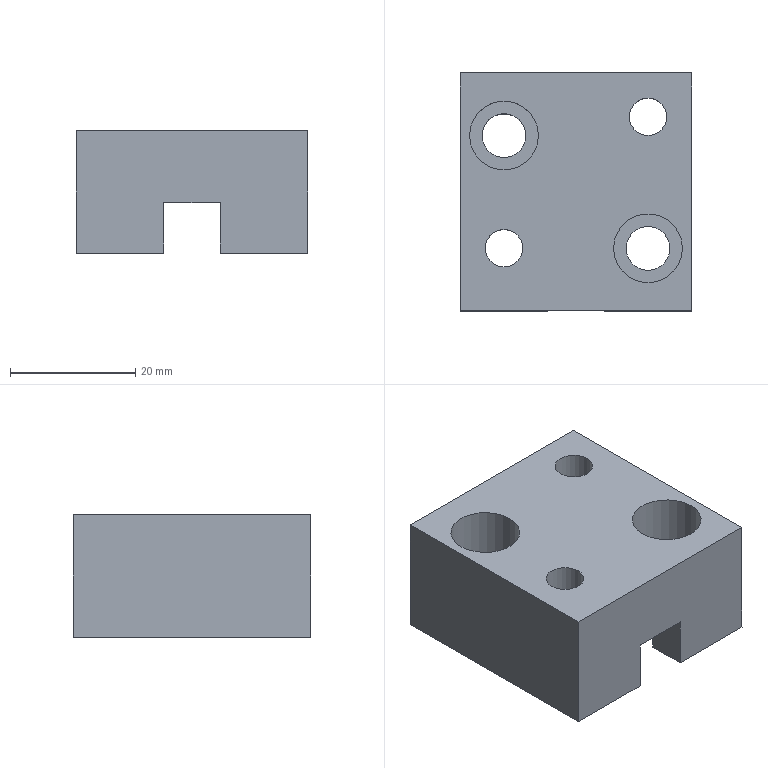Part | NX | features DIE-35 2 | 1 solid | 24 faces | box 37 x 38 x 19.5 mm | volume 18549 mm3 | plane 16 | cylinder 8 | commonest cylinder face diameters 3 x2 6 x2 7 x2 11 x2
STEP:
#1=CARTESIAN_POINT('',(2458.069,-966.622,879.216));
#2=VERTEX_POINT('',#1);
#3=CARTESIAN_POINT('',(2452.569,-966.622,879.216));
#4=DIRECTION('',(0.,0.,1.));
#5=DIRECTION('',(1.,0.,0.));
#6=AXIS2_PLACEMENT_3D('',#3,#4,#5);
#7=CIRCLE('',#6,5.5);
#8=EDGE_CURVE('',#2,#2,#7,.F.);
#9=ORIENTED_EDGE('',*,*,#8,.F.);
#10=EDGE_LOOP('',(#9));
#11=FACE_BOUND('',#10,.T.);
#12=CARTESIAN_POINT('',(2449.069,-966.622,879.216));
#13=VERTEX_POINT('',#12);
#14=CARTESIAN_POINT('',(2452.569,-966.622,879.216));
#15=DIRECTION('',(0.,0.,-1.));
#16=DIRECTION('',(-1.,0.,0.));
#17=AXIS2_PLACEMENT_3D('',#14,#15,#16);
#18=CIRCLE('',#17,3.5);
#19=EDGE_CURVE('',#13,#13,#18,.T.);
#20=ORIENTED_EDGE('',*,*,#19,.T.);
#21=EDGE_LOOP('',(#20));
#22=FACE_BOUND('',#21,.T.);
#23=CARTESIAN_POINT('',(2452.569,-966.622,879.216));
#24=DIRECTION('',(0.,0.,-1.));
#25=DIRECTION('',(-1.,0.,0.));
#26=AXIS2_PLACEMENT_3D('',#23,#24,#25);
#27=PLANE('',#26);
#28=ADVANCED_FACE('',(#11,#22),#27,.F.);
#29=CARTESIAN_POINT('',(2481.069,-984.622,879.216));
#30=VERTEX_POINT('',#29);
#31=CARTESIAN_POINT('',(2475.569,-984.622,879.216));
#32=DIRECTION('',(0.,0.,1.));
#33=DIRECTION('',(1.,0.,0.));
#34=AXIS2_PLACEMENT_3D('',#31,#32,#33);
#35=CIRCLE('',#34,5.5);
#36=EDGE_CURVE('',#30,#30,#35,.F.);
#37=ORIENTED_EDGE('',*,*,#36,.F.);
#38=EDGE_LOOP('',(#37));
#39=FACE_BOUND('',#38,.T.);
#40=CARTESIAN_POINT('',(2472.069,-984.622,879.216));
#41=VERTEX_POINT('',#40);
#42=CARTESIAN_POINT('',(2475.569,-984.622,879.216));
#43=DIRECTION('',(0.,0.,-1.));
#44=DIRECTION('',(-1.,0.,0.));
#45=AXIS2_PLACEMENT_3D('',#42,#43,#44);
#46=CIRCLE('',#45,3.5);
#47=EDGE_CURVE('',#41,#41,#46,.T.);
#48=ORIENTED_EDGE('',*,*,#47,.T.);
#49=EDGE_LOOP('',(#48));
#50=FACE_BOUND('',#49,.T.);
#51=CARTESIAN_POINT('',(2475.569,-984.622,879.216));
#52=DIRECTION('',(0.,0.,-1.));
#53=DIRECTION('',(-1.,0.,0.));
#54=AXIS2_PLACEMENT_3D('',#51,#52,#53);
#55=PLANE('',#54);
#56=ADVANCED_FACE('',(#39,#50),#55,.F.);
#57=CARTESIAN_POINT('',(2459.549,-956.622,868.716));
#58=VERTEX_POINT('',#57);
#59=CARTESIAN_POINT('',(2459.549,-956.622,885.266));
#60=VERTEX_POINT('',#59);
#61=CARTESIAN_POINT('',(2459.549,-956.622,878.466));
#62=DIRECTION('',(0.,0.,1.));
#63=VECTOR('',#62,1000.);
#64=LINE('',#61,#63);
#65=EDGE_CURVE('',#58,#60,#64,.T.);
#66=ORIENTED_EDGE('',*,*,#65,.T.);
#67=CARTESIAN_POINT('',(2459.549,-985.513,885.266));
#68=VERTEX_POINT('',#67);
#69=CARTESIAN_POINT('',(2459.549,-923.622,885.266));
#70=DIRECTION('',(0.,1.,0.));
#71=VECTOR('',#70,1000.);
#72=LINE('',#69,#71);
#73=EDGE_CURVE('',#68,#60,#72,.T.);
#74=ORIENTED_EDGE('',*,*,#73,.F.);
#75=CARTESIAN_POINT('',(2459.549,-985.513,868.716));
#76=VERTEX_POINT('',#75);
#77=CARTESIAN_POINT('',(2459.549,-985.513,885.266));
#78=DIRECTION('',(0.,0.,-1.));
#79=VECTOR('',#78,1000.);
#80=LINE('',#77,#79);
#81=EDGE_CURVE('',#68,#76,#80,.T.);
#82=ORIENTED_EDGE('',*,*,#81,.T.);
#83=CARTESIAN_POINT('',(2459.549,-849.622,868.716));
#84=DIRECTION('',(0.,-1.,0.));
#85=VECTOR('',#84,1000.);
#86=LINE('',#83,#85);
#87=EDGE_CURVE('',#58,#76,#86,.T.);
#88=ORIENTED_EDGE('',*,*,#87,.F.);
#89=EDGE_LOOP('',(#66,#74,#82,#88));
#90=FACE_BOUND('',#89,.T.);
#91=CARTESIAN_POINT('',(2459.549,-923.622,868.716));
#92=DIRECTION('',(-1.,0.,0.));
#93=DIRECTION('',(0.,0.,-1.));
#94=AXIS2_PLACEMENT_3D('',#91,#92,#93);
#95=PLANE('',#94);
#96=ADVANCED_FACE('',(#90),#95,.F.);
#97=CARTESIAN_POINT('',(2478.569,-963.622,868.716));
#98=VERTEX_POINT('',#97);
#99=CARTESIAN_POINT('',(2475.569,-963.622,868.716));
#100=DIRECTION('',(0.,0.,1.));
#101=DIRECTION('',(1.,0.,0.));
#102=AXIS2_PLACEMENT_3D('',#99,#100,#101);
#103=CIRCLE('',#102,3.);
#104=EDGE_CURVE('',#98,#98,#103,.T.);
#105=ORIENTED_EDGE('',*,*,#104,.T.);
#106=EDGE_LOOP('',(#105));
#107=FACE_BOUND('',#106,.T.);
#108=CARTESIAN_POINT('',(2479.069,-984.622,868.716));
#109=VERTEX_POINT('',#108);
#110=CARTESIAN_POINT('',(2475.569,-984.622,868.716));
#111=DIRECTION('',(0.,0.,1.));
#112=DIRECTION('',(1.,0.,0.));
#113=AXIS2_PLACEMENT_3D('',#110,#111,#112);
#114=CIRCLE('',#113,3.5);
#115=EDGE_CURVE('',#109,#109,#114,.T.);
#116=ORIENTED_EDGE('',*,*,#115,.T.);
#117=EDGE_LOOP('',(#116));
#118=FACE_BOUND('',#117,.T.);
#119=CARTESIAN_POINT('',(2468.589,-956.622,868.716));
#120=VERTEX_POINT('',#119);
#121=CARTESIAN_POINT('',(2482.569,-956.622,868.716));
#122=VERTEX_POINT('',#121);
#123=CARTESIAN_POINT('',(2464.069,-956.622,868.716));
#124=DIRECTION('',(1.,0.,0.));
#125=VECTOR('',#124,1000.);
#126=LINE('',#123,#125);
#127=EDGE_CURVE('',#120,#122,#126,.T.);
#128=ORIENTED_EDGE('',*,*,#127,.T.);
#129=CARTESIAN_POINT('',(2482.569,-994.622,868.716));
#130=VERTEX_POINT('',#129);
#131=CARTESIAN_POINT('',(2482.569,-989.622,868.716));
#132=DIRECTION('',(0.,-1.,0.));
#133=VECTOR('',#132,1000.);
#134=LINE('',#131,#133);
#135=EDGE_CURVE('',#122,#130,#134,.T.);
#136=ORIENTED_EDGE('',*,*,#135,.T.);
#137=CARTESIAN_POINT('',(2468.589,-994.622,868.716));
#138=VERTEX_POINT('',#137);
#139=CARTESIAN_POINT('',(2529.569,-994.622,868.716));
#140=DIRECTION('',(1.,0.,0.));
#141=VECTOR('',#140,1000.);
#142=LINE('',#139,#141);
#143=EDGE_CURVE('',#138,#130,#142,.T.);
#144=ORIENTED_EDGE('',*,*,#143,.F.);
#145=CARTESIAN_POINT('',(2468.589,-988.438,868.716));
#146=VERTEX_POINT('',#145);
#147=CARTESIAN_POINT('',(2468.589,-849.622,868.716));
#148=DIRECTION('',(0.,1.,0.));
#149=VECTOR('',#148,1000.);
#150=LINE('',#147,#149);
#151=EDGE_CURVE('',#138,#146,#150,.T.);
#152=ORIENTED_EDGE('',*,*,#151,.T.);
#153=CARTESIAN_POINT('',(2468.589,-985.513,868.716));
#154=VERTEX_POINT('',#153);
#155=CARTESIAN_POINT('',(2468.922,-986.976,868.716));
#156=DIRECTION('',(0.,0.,1.));
#157=DIRECTION('',(1.,0.,0.));
#158=AXIS2_PLACEMENT_3D('',#155,#156,#157);
#159=CIRCLE('',#158,1.5);
#160=EDGE_CURVE('',#146,#154,#159,.T.);
#161=ORIENTED_EDGE('',*,*,#160,.T.);
#162=CARTESIAN_POINT('',(2468.589,-849.622,868.716));
#163=DIRECTION('',(0.,1.,0.));
#164=VECTOR('',#163,1000.);
#165=LINE('',#162,#164);
#166=EDGE_CURVE('',#154,#120,#165,.T.);
#167=ORIENTED_EDGE('',*,*,#166,.T.);
#168=EDGE_LOOP('',(#128,#136,#144,#152,#161,#167));
#169=FACE_BOUND('',#168,.T.);
#170=CARTESIAN_POINT('',(2529.569,-849.622,868.716));
#171=DIRECTION('',(0.,0.,1.));
#172=DIRECTION('',(-1.,0.,0.));
#173=AXIS2_PLACEMENT_3D('',#170,#171,#172);
#174=PLANE('',#173);
#175=ADVANCED_FACE('',(#107,#118,#169),#174,.F.);
#176=CARTESIAN_POINT('',(2478.569,-963.622,888.216));
#177=VERTEX_POINT('',#176);
#178=CARTESIAN_POINT('',(2475.569,-963.622,888.216));
#179=DIRECTION('',(0.,0.,1.));
#180=DIRECTION('',(1.,0.,0.));
#181=AXIS2_PLACEMENT_3D('',#178,#179,#180);
#182=CIRCLE('',#181,3.);
#183=EDGE_CURVE('',#177,#177,#182,.F.);
#184=ORIENTED_EDGE('',*,*,#183,.T.);
#185=EDGE_LOOP('',(#184));
#186=FACE_BOUND('',#185,.T.);
#187=CARTESIAN_POINT('',(2455.569,-984.622,888.216));
#188=VERTEX_POINT('',#187);
#189=CARTESIAN_POINT('',(2452.569,-984.622,888.216));
#190=DIRECTION('',(0.,0.,1.));
#191=DIRECTION('',(1.,0.,0.));
#192=AXIS2_PLACEMENT_3D('',#189,#190,#191);
#193=CIRCLE('',#192,3.);
#194=EDGE_CURVE('',#188,#188,#193,.F.);
#195=ORIENTED_EDGE('',*,*,#194,.T.);
#196=EDGE_LOOP('',(#195));
#197=FACE_BOUND('',#196,.T.);
#198=CARTESIAN_POINT('',(2481.069,-984.622,888.216));
#199=VERTEX_POINT('',#198);
#200=CARTESIAN_POINT('',(2475.569,-984.622,888.216));
#201=DIRECTION('',(0.,0.,-1.));
#202=DIRECTION('',(1.,0.,0.));
#203=AXIS2_PLACEMENT_3D('',#200,#201,#202);
#204=CIRCLE('',#203,5.5);
#205=EDGE_CURVE('',#199,#199,#204,.T.);
#206=ORIENTED_EDGE('',*,*,#205,.T.);
#207=EDGE_LOOP('',(#206));
#208=FACE_BOUND('',#207,.T.);
#209=CARTESIAN_POINT('',(2458.069,-966.622,888.216));
#210=VERTEX_POINT('',#209);
#211=CARTESIAN_POINT('',(2452.569,-966.622,888.216));
#212=DIRECTION('',(0.,0.,-1.));
#213=DIRECTION('',(1.,0.,0.));
#214=AXIS2_PLACEMENT_3D('',#211,#212,#213);
#215=CIRCLE('',#214,5.5);
#216=EDGE_CURVE('',#210,#210,#215,.T.);
#217=ORIENTED_EDGE('',*,*,#216,.T.);
#218=EDGE_LOOP('',(#217));
#219=FACE_BOUND('',#218,.T.);
#220=CARTESIAN_POINT('',(2482.569,-956.622,888.216));
#221=VERTEX_POINT('',#220);
#222=CARTESIAN_POINT('',(2482.569,-994.622,888.216));
#223=VERTEX_POINT('',#222);
#224=CARTESIAN_POINT('',(2482.569,-989.622,888.216));
#225=DIRECTION('',(0.,-1.,0.));
#226=VECTOR('',#225,1000.);
#227=LINE('',#224,#226);
#228=EDGE_CURVE('',#221,#223,#227,.T.);
#229=ORIENTED_EDGE('',*,*,#228,.F.);
#230=CARTESIAN_POINT('',(2445.569,-956.622,888.216));
#231=VERTEX_POINT('',#230);
#232=CARTESIAN_POINT('',(2464.069,-956.622,888.216));
#233=DIRECTION('',(1.,0.,0.));
#234=VECTOR('',#233,1000.);
#235=LINE('',#232,#234);
#236=EDGE_CURVE('',#231,#221,#235,.T.);
#237=ORIENTED_EDGE('',*,*,#236,.F.);
#238=CARTESIAN_POINT('',(2445.569,-994.622,888.216));
#239=VERTEX_POINT('',#238);
#240=CARTESIAN_POINT('',(2445.569,-989.622,888.216));
#241=DIRECTION('',(0.,1.,0.));
#242=VECTOR('',#241,1000.);
#243=LINE('',#240,#242);
#244=EDGE_CURVE('',#239,#231,#243,.T.);
#245=ORIENTED_EDGE('',*,*,#244,.F.);
#246=CARTESIAN_POINT('',(2691.569,-994.622,888.216));
#247=DIRECTION('',(-1.,0.,0.));
#248=VECTOR('',#247,1000.);
#249=LINE('',#246,#248);
#250=EDGE_CURVE('',#223,#239,#249,.T.);
#251=ORIENTED_EDGE('',*,*,#250,.F.);
#252=EDGE_LOOP('',(#229,#237,#245,#251));
#253=FACE_BOUND('',#252,.T.);
#254=CARTESIAN_POINT('',(2463.569,-989.622,888.216));
#255=DIRECTION('',(0.,0.,1.));
#256=DIRECTION('',(-1.,0.,0.));
#257=AXIS2_PLACEMENT_3D('',#254,#255,#256);
#258=PLANE('',#257);
#259=ADVANCED_FACE('',(#186,#197,#208,#219,#253),#258,.T.);
#260=ORIENTED_EDGE('',*,*,#244,.T.);
#261=CARTESIAN_POINT('',(2445.569,-956.622,868.716));
#262=VERTEX_POINT('',#261);
#263=CARTESIAN_POINT('',(2445.569,-956.622,860.716));
#264=DIRECTION('',(0.,0.,-1.));
#265=VECTOR('',#264,1000.);
#266=LINE('',#263,#265);
#267=EDGE_CURVE('',#231,#262,#266,.T.);
#268=ORIENTED_EDGE('',*,*,#267,.T.);
#269=CARTESIAN_POINT('',(2445.569,-994.622,868.716));
#270=VERTEX_POINT('',#269);
#271=CARTESIAN_POINT('',(2445.569,-989.622,868.716));
#272=DIRECTION('',(0.,1.,0.));
#273=VECTOR('',#272,1000.);
#274=LINE('',#271,#273);
#275=EDGE_CURVE('',#270,#262,#274,.T.);
#276=ORIENTED_EDGE('',*,*,#275,.F.);
#277=CARTESIAN_POINT('',(2445.569,-994.622,860.716));
#278=DIRECTION('',(0.,0.,1.));
#279=VECTOR('',#278,1000.);
#280=LINE('',#277,#279);
#281=EDGE_CURVE('',#270,#239,#280,.T.);
#282=ORIENTED_EDGE('',*,*,#281,.T.);
#283=EDGE_LOOP('',(#260,#268,#276,#282));
#284=FACE_BOUND('',#283,.T.);
#285=CARTESIAN_POINT('',(2445.569,-989.622,860.716));
#286=DIRECTION('',(-1.,0.,0.));
#287=DIRECTION('',(0.,0.,-1.));
#288=AXIS2_PLACEMENT_3D('',#285,#286,#287);
#289=PLANE('',#288);
#290=ADVANCED_FACE('',(#284),#289,.T.);
#291=ORIENTED_EDGE('',*,*,#135,.F.);
#292=CARTESIAN_POINT('',(2482.569,-956.622,878.466));
#293=DIRECTION('',(0.,0.,-1.));
#294=VECTOR('',#293,1000.);
#295=LINE('',#292,#294);
#296=EDGE_CURVE('',#221,#122,#295,.T.);
#297=ORIENTED_EDGE('',*,*,#296,.F.);
#298=ORIENTED_EDGE('',*,*,#228,.T.);
#299=CARTESIAN_POINT('',(2482.569,-994.622,803.716));
#300=DIRECTION('',(0.,0.,1.));
#301=VECTOR('',#300,1000.);
#302=LINE('',#299,#301);
#303=EDGE_CURVE('',#130,#223,#302,.T.);
#304=ORIENTED_EDGE('',*,*,#303,.F.);
#305=EDGE_LOOP('',(#291,#297,#298,#304));
#306=FACE_BOUND('',#305,.T.);
#307=CARTESIAN_POINT('',(2482.569,-989.622,860.716));
#308=DIRECTION('',(1.,0.,0.));
#309=DIRECTION('',(0.,0.,1.));
#310=AXIS2_PLACEMENT_3D('',#307,#308,#309);
#311=PLANE('',#310);
#312=ADVANCED_FACE('',(#306),#311,.T.);
#313=CARTESIAN_POINT('',(2455.569,-984.622,868.716));
#314=VERTEX_POINT('',#313);
#315=CARTESIAN_POINT('',(2452.569,-984.622,868.716));
#316=DIRECTION('',(0.,0.,1.));
#317=DIRECTION('',(1.,0.,0.));
#318=AXIS2_PLACEMENT_3D('',#315,#316,#317);
#319=CIRCLE('',#318,3.);
#320=EDGE_CURVE('',#314,#314,#319,.T.);
#321=ORIENTED_EDGE('',*,*,#320,.T.);
#322=EDGE_LOOP('',(#321));
#323=FACE_BOUND('',#322,.T.);
#324=CARTESIAN_POINT('',(2456.069,-966.622,868.716));
#325=VERTEX_POINT('',#324);
#326=CARTESIAN_POINT('',(2452.569,-966.622,868.716));
#327=DIRECTION('',(0.,0.,1.));
#328=DIRECTION('',(1.,0.,0.));
#329=AXIS2_PLACEMENT_3D('',#326,#327,#328);
#330=CIRCLE('',#329,3.5);
#331=EDGE_CURVE('',#325,#325,#330,.T.);
#332=ORIENTED_EDGE('',*,*,#331,.T.);
#333=EDGE_LOOP('',(#332));
#334=FACE_BOUND('',#333,.T.);
#335=CARTESIAN_POINT('',(2464.069,-956.622,868.716));
#336=DIRECTION('',(1.,0.,0.));
#337=VECTOR('',#336,1000.);
#338=LINE('',#335,#337);
#339=EDGE_CURVE('',#262,#58,#338,.T.);
#340=ORIENTED_EDGE('',*,*,#339,.T.);
#341=ORIENTED_EDGE('',*,*,#87,.T.);
#342=CARTESIAN_POINT('',(2459.549,-988.438,868.716));
#343=VERTEX_POINT('',#342);
#344=CARTESIAN_POINT('',(2459.215,-986.976,868.716));
#345=DIRECTION('',(0.,0.,1.));
#346=DIRECTION('',(1.,0.,0.));
#347=AXIS2_PLACEMENT_3D('',#344,#345,#346);
#348=CIRCLE('',#347,1.5);
#349=EDGE_CURVE('',#76,#343,#348,.T.);
#350=ORIENTED_EDGE('',*,*,#349,.T.);
#351=CARTESIAN_POINT('',(2459.549,-994.622,868.716));
#352=VERTEX_POINT('',#351);
#353=CARTESIAN_POINT('',(2459.549,-849.622,868.716));
#354=DIRECTION('',(0.,-1.,0.));
#355=VECTOR('',#354,1000.);
#356=LINE('',#353,#355);
#357=EDGE_CURVE('',#343,#352,#356,.T.);
#358=ORIENTED_EDGE('',*,*,#357,.T.);
#359=CARTESIAN_POINT('',(2529.569,-994.622,868.716));
#360=DIRECTION('',(1.,0.,0.));
#361=VECTOR('',#360,1000.);
#362=LINE('',#359,#361);
#363=EDGE_CURVE('',#270,#352,#362,.T.);
#364=ORIENTED_EDGE('',*,*,#363,.F.);
#365=ORIENTED_EDGE('',*,*,#275,.T.);
#366=EDGE_LOOP('',(#340,#341,#350,#358,#364,#365));
#367=FACE_BOUND('',#366,.T.);
#368=CARTESIAN_POINT('',(2529.569,-849.622,868.716));
#369=DIRECTION('',(0.,0.,1.));
#370=DIRECTION('',(-1.,0.,0.));
#371=AXIS2_PLACEMENT_3D('',#368,#369,#370);
#372=PLANE('',#371);
#373=ADVANCED_FACE('',(#323,#334,#367),#372,.F.);
#374=CARTESIAN_POINT('',(2468.589,-956.622,885.266));
#375=VERTEX_POINT('',#374);
#376=CARTESIAN_POINT('',(2468.589,-956.622,878.466));
#377=DIRECTION('',(0.,0.,-1.));
#378=VECTOR('',#377,1000.);
#379=LINE('',#376,#378);
#380=EDGE_CURVE('',#375,#120,#379,.T.);
#381=ORIENTED_EDGE('',*,*,#380,.T.);
#382=ORIENTED_EDGE('',*,*,#166,.F.);
#383=CARTESIAN_POINT('',(2468.589,-985.513,885.266));
#384=VERTEX_POINT('',#383);
#385=CARTESIAN_POINT('',(2468.589,-985.513,885.266));
#386=DIRECTION('',(0.,0.,-1.));
#387=VECTOR('',#386,1000.);
#388=LINE('',#385,#387);
#389=EDGE_CURVE('',#154,#384,#388,.F.);
#390=ORIENTED_EDGE('',*,*,#389,.T.);
#391=CARTESIAN_POINT('',(2468.589,-923.622,885.266));
#392=DIRECTION('',(0.,-1.,0.));
#393=VECTOR('',#392,1000.);
#394=LINE('',#391,#393);
#395=EDGE_CURVE('',#375,#384,#394,.T.);
#396=ORIENTED_EDGE('',*,*,#395,.F.);
#397=EDGE_LOOP('',(#381,#382,#390,#396));
#398=FACE_BOUND('',#397,.T.);
#399=CARTESIAN_POINT('',(2468.589,-923.622,868.716));
#400=DIRECTION('',(1.,0.,0.));
#401=DIRECTION('',(0.,0.,1.));
#402=AXIS2_PLACEMENT_3D('',#399,#400,#401);
#403=PLANE('',#402);
#404=ADVANCED_FACE('',(#398),#403,.F.);
#405=CARTESIAN_POINT('',(2464.069,-956.622,885.266));
#406=DIRECTION('',(1.,0.,0.));
#407=VECTOR('',#406,1000.);
#408=LINE('',#405,#407);
#409=EDGE_CURVE('',#60,#375,#408,.T.);
#410=ORIENTED_EDGE('',*,*,#409,.T.);
#411=ORIENTED_EDGE('',*,*,#395,.T.);
#412=CARTESIAN_POINT('',(2467.465,-986.622,885.266));
#413=VERTEX_POINT('',#412);
#414=CARTESIAN_POINT('',(2468.922,-986.976,885.266));
#415=DIRECTION('',(0.,0.,-1.));
#416=DIRECTION('',(1.,0.,0.));
#417=AXIS2_PLACEMENT_3D('',#414,#415,#416);
#418=CIRCLE('',#417,1.5);
#419=EDGE_CURVE('',#384,#413,#418,.T.);
#420=ORIENTED_EDGE('',*,*,#419,.T.);
#421=CARTESIAN_POINT('',(2460.673,-986.622,885.266));
#422=VERTEX_POINT('',#421);
#423=CARTESIAN_POINT('',(2465.569,-986.622,885.266));
#424=DIRECTION('',(-1.,0.,0.));
#425=VECTOR('',#424,1000.);
#426=LINE('',#423,#425);
#427=EDGE_CURVE('',#413,#422,#426,.T.);
#428=ORIENTED_EDGE('',*,*,#427,.T.);
#429=CARTESIAN_POINT('',(2459.215,-986.976,885.266));
#430=DIRECTION('',(0.,0.,-1.));
#431=DIRECTION('',(1.,0.,0.));
#432=AXIS2_PLACEMENT_3D('',#429,#430,#431);
#433=CIRCLE('',#432,1.5);
#434=EDGE_CURVE('',#422,#68,#433,.T.);
#435=ORIENTED_EDGE('',*,*,#434,.T.);
#436=ORIENTED_EDGE('',*,*,#73,.T.);
#437=EDGE_LOOP('',(#410,#411,#420,#428,#435,#436));
#438=FACE_BOUND('',#437,.T.);
#439=CARTESIAN_POINT('',(2465.569,-923.622,885.266));
#440=DIRECTION('',(0.,0.,1.));
#441=DIRECTION('',(-1.,0.,0.));
#442=AXIS2_PLACEMENT_3D('',#439,#440,#441);
#443=PLANE('',#442);
#444=ADVANCED_FACE('',(#438),#443,.F.);
#445=CARTESIAN_POINT('',(2468.589,-994.622,876.736));
#446=VERTEX_POINT('',#445);
#447=CARTESIAN_POINT('',(2468.589,-988.438,876.736));
#448=VERTEX_POINT('',#447);
#449=CARTESIAN_POINT('',(2468.589,-948.622,876.736));
#450=DIRECTION('',(0.,1.,0.));
#451=VECTOR('',#450,1000.);
#452=LINE('',#449,#451);
#453=EDGE_CURVE('',#446,#448,#452,.T.);
#454=ORIENTED_EDGE('',*,*,#453,.T.);
#455=CARTESIAN_POINT('',(2468.589,-988.438,885.266));
#456=DIRECTION('',(0.,0.,-1.));
#457=VECTOR('',#456,1000.);
#458=LINE('',#455,#457);
#459=EDGE_CURVE('',#448,#146,#458,.T.);
#460=ORIENTED_EDGE('',*,*,#459,.T.);
#461=ORIENTED_EDGE('',*,*,#151,.F.);
#462=CARTESIAN_POINT('',(2468.589,-994.622,803.716));
#463=DIRECTION('',(0.,0.,1.));
#464=VECTOR('',#463,1000.);
#465=LINE('',#462,#464);
#466=EDGE_CURVE('',#138,#446,#465,.T.);
#467=ORIENTED_EDGE('',*,*,#466,.T.);
#468=EDGE_LOOP('',(#454,#460,#461,#467));
#469=FACE_BOUND('',#468,.T.);
#470=CARTESIAN_POINT('',(2468.589,-923.622,868.716));
#471=DIRECTION('',(1.,0.,0.));
#472=DIRECTION('',(0.,0.,1.));
#473=AXIS2_PLACEMENT_3D('',#470,#471,#472);
#474=PLANE('',#473);
#475=ADVANCED_FACE('',(#469),#474,.F.);
#476=CARTESIAN_POINT('',(2459.549,-988.438,876.736));
#477=VERTEX_POINT('',#476);
#478=CARTESIAN_POINT('',(2459.549,-994.622,876.736));
#479=VERTEX_POINT('',#478);
#480=CARTESIAN_POINT('',(2459.549,-948.622,876.736));
#481=DIRECTION('',(0.,-1.,0.));
#482=VECTOR('',#481,1000.);
#483=LINE('',#480,#482);
#484=EDGE_CURVE('',#477,#479,#483,.T.);
#485=ORIENTED_EDGE('',*,*,#484,.F.);
#486=CARTESIAN_POINT('',(2460.673,-986.622,876.736));
#487=VERTEX_POINT('',#486);
#488=CARTESIAN_POINT('',(2459.215,-986.976,876.736));
#489=DIRECTION('',(0.,0.,1.));
#490=DIRECTION('',(1.,0.,0.));
#491=AXIS2_PLACEMENT_3D('',#488,#489,#490);
#492=CIRCLE('',#491,1.5);
#493=EDGE_CURVE('',#477,#487,#492,.T.);
#494=ORIENTED_EDGE('',*,*,#493,.T.);
#495=CARTESIAN_POINT('',(2467.465,-986.622,876.736));
#496=VERTEX_POINT('',#495);
#497=CARTESIAN_POINT('',(2463.569,-986.622,876.736));
#498=DIRECTION('',(-1.,0.,0.));
#499=VECTOR('',#498,1000.);
#500=LINE('',#497,#499);
#501=EDGE_CURVE('',#496,#487,#500,.T.);
#502=ORIENTED_EDGE('',*,*,#501,.F.);
#503=CARTESIAN_POINT('',(2468.922,-986.976,876.736));
#504=DIRECTION('',(0.,0.,1.));
#505=DIRECTION('',(1.,0.,0.));
#506=AXIS2_PLACEMENT_3D('',#503,#504,#505);
#507=CIRCLE('',#506,1.5);
#508=EDGE_CURVE('',#496,#448,#507,.T.);
#509=ORIENTED_EDGE('',*,*,#508,.T.);
#510=ORIENTED_EDGE('',*,*,#453,.F.);
#511=CARTESIAN_POINT('',(2691.569,-994.622,876.736));
#512=DIRECTION('',(-1.,0.,0.));
#513=VECTOR('',#512,1000.);
#514=LINE('',#511,#513);
#515=EDGE_CURVE('',#446,#479,#514,.T.);
#516=ORIENTED_EDGE('',*,*,#515,.T.);
#517=EDGE_LOOP('',(#485,#494,#502,#509,#510,#516));
#518=FACE_BOUND('',#517,.T.);
#519=CARTESIAN_POINT('',(2463.569,-948.622,876.736));
#520=DIRECTION('',(0.,0.,1.));
#521=DIRECTION('',(-1.,0.,0.));
#522=AXIS2_PLACEMENT_3D('',#519,#520,#521);
#523=PLANE('',#522);
#524=ADVANCED_FACE('',(#518),#523,.F.);
#525=ORIENTED_EDGE('',*,*,#515,.F.);
#526=ORIENTED_EDGE('',*,*,#466,.F.);
#527=ORIENTED_EDGE('',*,*,#143,.T.);
#528=ORIENTED_EDGE('',*,*,#303,.T.);
#529=ORIENTED_EDGE('',*,*,#250,.T.);
#530=ORIENTED_EDGE('',*,*,#281,.F.);
#531=ORIENTED_EDGE('',*,*,#363,.T.);
#532=CARTESIAN_POINT('',(2459.549,-994.622,803.716));
#533=DIRECTION('',(0.,0.,-1.));
#534=VECTOR('',#533,1000.);
#535=LINE('',#532,#534);
#536=EDGE_CURVE('',#479,#352,#535,.T.);
#537=ORIENTED_EDGE('',*,*,#536,.F.);
#538=EDGE_LOOP('',(#525,#526,#527,#528,#529,#530,#531,#537));
#539=FACE_BOUND('',#538,.T.);
#540=CARTESIAN_POINT('',(2691.569,-994.622,803.716));
#541=DIRECTION('',(0.,-1.,0.));
#542=DIRECTION('',(0.,0.,-1.));
#543=AXIS2_PLACEMENT_3D('',#540,#541,#542);
#544=PLANE('',#543);
#545=ADVANCED_FACE('',(#539),#544,.T.);
#546=ORIENTED_EDGE('',*,*,#357,.F.);
#547=CARTESIAN_POINT('',(2459.549,-988.438,885.266));
#548=DIRECTION('',(0.,0.,-1.));
#549=VECTOR('',#548,1000.);
#550=LINE('',#547,#549);
#551=EDGE_CURVE('',#343,#477,#550,.F.);
#552=ORIENTED_EDGE('',*,*,#551,.T.);
#553=ORIENTED_EDGE('',*,*,#484,.T.);
#554=ORIENTED_EDGE('',*,*,#536,.T.);
#555=EDGE_LOOP('',(#546,#552,#553,#554));
#556=FACE_BOUND('',#555,.T.);
#557=CARTESIAN_POINT('',(2459.549,-923.622,868.716));
#558=DIRECTION('',(-1.,0.,0.));
#559=DIRECTION('',(0.,0.,-1.));
#560=AXIS2_PLACEMENT_3D('',#557,#558,#559);
#561=PLANE('',#560);
#562=ADVANCED_FACE('',(#556),#561,.F.);
#563=CARTESIAN_POINT('',(2460.673,-986.622,885.266));
#564=DIRECTION('',(0.,0.,-1.));
#565=VECTOR('',#564,1000.);
#566=LINE('',#563,#565);
#567=EDGE_CURVE('',#422,#487,#566,.T.);
#568=ORIENTED_EDGE('',*,*,#567,.F.);
#569=ORIENTED_EDGE('',*,*,#427,.F.);
#570=CARTESIAN_POINT('',(2467.465,-986.622,885.266));
#571=DIRECTION('',(0.,0.,1.));
#572=VECTOR('',#571,1000.);
#573=LINE('',#570,#572);
#574=EDGE_CURVE('',#496,#413,#573,.T.);
#575=ORIENTED_EDGE('',*,*,#574,.F.);
#576=ORIENTED_EDGE('',*,*,#501,.T.);
#577=EDGE_LOOP('',(#568,#569,#575,#576));
#578=FACE_BOUND('',#577,.T.);
#579=CARTESIAN_POINT('',(2463.569,-986.622,860.716));
#580=DIRECTION('',(0.,1.,0.));
#581=DIRECTION('',(0.,0.,-1.));
#582=AXIS2_PLACEMENT_3D('',#579,#580,#581);
#583=PLANE('',#582);
#584=ADVANCED_FACE('',(#578),#583,.T.);
#585=ORIENTED_EDGE('',*,*,#160,.F.);
#586=ORIENTED_EDGE('',*,*,#459,.F.);
#587=ORIENTED_EDGE('',*,*,#508,.F.);
#588=ORIENTED_EDGE('',*,*,#574,.T.);
#589=ORIENTED_EDGE('',*,*,#419,.F.);
#590=ORIENTED_EDGE('',*,*,#389,.F.);
#591=EDGE_LOOP('',(#585,#586,#587,#588,#589,#590));
#592=FACE_BOUND('',#591,.T.);
#593=CARTESIAN_POINT('',(2468.922,-986.976,885.266));
#594=DIRECTION('',(0.,0.,-1.));
#595=DIRECTION('',(-1.,0.,0.));
#596=AXIS2_PLACEMENT_3D('',#593,#594,#595);
#597=CYLINDRICAL_SURFACE('',#596,1.5);
#598=ADVANCED_FACE('',(#592),#597,.F.);
#599=ORIENTED_EDGE('',*,*,#434,.F.);
#600=ORIENTED_EDGE('',*,*,#567,.T.);
#601=ORIENTED_EDGE('',*,*,#493,.F.);
#602=ORIENTED_EDGE('',*,*,#551,.F.);
#603=ORIENTED_EDGE('',*,*,#349,.F.);
#604=ORIENTED_EDGE('',*,*,#81,.F.);
#605=EDGE_LOOP('',(#599,#600,#601,#602,#603,#604));
#606=FACE_BOUND('',#605,.T.);
#607=CARTESIAN_POINT('',(2459.215,-986.976,885.266));
#608=DIRECTION('',(0.,0.,-1.));
#609=DIRECTION('',(-1.,0.,0.));
#610=AXIS2_PLACEMENT_3D('',#607,#608,#609);
#611=CYLINDRICAL_SURFACE('',#610,1.5);
#612=ADVANCED_FACE('',(#606),#611,.F.);
#613=ORIENTED_EDGE('',*,*,#236,.T.);
#614=ORIENTED_EDGE('',*,*,#296,.T.);
#615=ORIENTED_EDGE('',*,*,#127,.F.);
#616=ORIENTED_EDGE('',*,*,#380,.F.);
#617=ORIENTED_EDGE('',*,*,#409,.F.);
#618=ORIENTED_EDGE('',*,*,#65,.F.);
#619=ORIENTED_EDGE('',*,*,#339,.F.);
#620=ORIENTED_EDGE('',*,*,#267,.F.);
#621=EDGE_LOOP('',(#613,#614,#615,#616,#617,#618,#619,#620));
#622=FACE_BOUND('',#621,.T.);
#623=CARTESIAN_POINT('',(2464.069,-956.622,878.466));
#624=DIRECTION('',(0.,1.,0.));
#625=DIRECTION('',(0.,0.,-1.));
#626=AXIS2_PLACEMENT_3D('',#623,#624,#625);
#627=PLANE('',#626);
#628=ADVANCED_FACE('',(#622),#627,.T.);
#629=ORIENTED_EDGE('',*,*,#8,.T.);
#630=EDGE_LOOP('',(#629));
#631=FACE_BOUND('',#630,.T.);
#632=ORIENTED_EDGE('',*,*,#216,.F.);
#633=EDGE_LOOP('',(#632));
#634=FACE_BOUND('',#633,.T.);
#635=CARTESIAN_POINT('',(2452.569,-966.622,888.216));
#636=DIRECTION('',(0.,0.,-1.));
#637=DIRECTION('',(1.,0.,0.));
#638=AXIS2_PLACEMENT_3D('',#635,#636,#637);
#639=CYLINDRICAL_SURFACE('',#638,5.5);
#640=ADVANCED_FACE('',(#631,#634),#639,.F.);
#641=ORIENTED_EDGE('',*,*,#331,.F.);
#642=EDGE_LOOP('',(#641));
#643=FACE_BOUND('',#642,.T.);
#644=ORIENTED_EDGE('',*,*,#19,.F.);
#645=EDGE_LOOP('',(#644));
#646=FACE_BOUND('',#645,.T.);
#647=CARTESIAN_POINT('',(2452.569,-966.622,888.216));
#648=DIRECTION('',(0.,0.,-1.));
#649=DIRECTION('',(1.,0.,0.));
#650=AXIS2_PLACEMENT_3D('',#647,#648,#649);
#651=CYLINDRICAL_SURFACE('',#650,3.5);
#652=ADVANCED_FACE('',(#643,#646),#651,.F.);
#653=ORIENTED_EDGE('',*,*,#36,.T.);
#654=EDGE_LOOP('',(#653));
#655=FACE_BOUND('',#654,.T.);
#656=ORIENTED_EDGE('',*,*,#205,.F.);
#657=EDGE_LOOP('',(#656));
#658=FACE_BOUND('',#657,.T.);
#659=CARTESIAN_POINT('',(2475.569,-984.622,888.216));
#660=DIRECTION('',(0.,0.,-1.));
#661=DIRECTION('',(1.,0.,0.));
#662=AXIS2_PLACEMENT_3D('',#659,#660,#661);
#663=CYLINDRICAL_SURFACE('',#662,5.5);
#664=ADVANCED_FACE('',(#655,#658),#663,.F.);
#665=ORIENTED_EDGE('',*,*,#115,.F.);
#666=EDGE_LOOP('',(#665));
#667=FACE_BOUND('',#666,.T.);
#668=ORIENTED_EDGE('',*,*,#47,.F.);
#669=EDGE_LOOP('',(#668));
#670=FACE_BOUND('',#669,.T.);
#671=CARTESIAN_POINT('',(2475.569,-984.622,888.216));
#672=DIRECTION('',(0.,0.,-1.));
#673=DIRECTION('',(1.,0.,0.));
#674=AXIS2_PLACEMENT_3D('',#671,#672,#673);
#675=CYLINDRICAL_SURFACE('',#674,3.5);
#676=ADVANCED_FACE('',(#667,#670),#675,.F.);
#677=ORIENTED_EDGE('',*,*,#194,.F.);
#678=EDGE_LOOP('',(#677));
#679=FACE_BOUND('',#678,.T.);
#680=ORIENTED_EDGE('',*,*,#320,.F.);
#681=EDGE_LOOP('',(#680));
#682=FACE_BOUND('',#681,.T.);
#683=CARTESIAN_POINT('',(2452.569,-984.622,888.216));
#684=DIRECTION('',(0.,0.,-1.));
#685=DIRECTION('',(1.,0.,0.));
#686=AXIS2_PLACEMENT_3D('',#683,#684,#685);
#687=CYLINDRICAL_SURFACE('',#686,3.);
#688=ADVANCED_FACE('',(#679,#682),#687,.F.);
#689=ORIENTED_EDGE('',*,*,#183,.F.);
#690=EDGE_LOOP('',(#689));
#691=FACE_BOUND('',#690,.T.);
#692=ORIENTED_EDGE('',*,*,#104,.F.);
#693=EDGE_LOOP('',(#692));
#694=FACE_BOUND('',#693,.T.);
#695=CARTESIAN_POINT('',(2475.569,-963.622,888.216));
#696=DIRECTION('',(0.,0.,-1.));
#697=DIRECTION('',(1.,0.,0.));
#698=AXIS2_PLACEMENT_3D('',#695,#696,#697);
#699=CYLINDRICAL_SURFACE('',#698,3.);
#700=ADVANCED_FACE('',(#691,#694),#699,.F.);
#701=CLOSED_SHELL('',(#28,#56,#96,#175,#259,#290,#312,#373,#404,#444,#475,#524,#545,#562,#584,#598,#612,#628,#640,#652,#664,#676,#688,#700));
#702=MANIFOLD_SOLID_BREP('',#701);
#703=(LENGTH_UNIT()NAMED_UNIT(*)SI_UNIT(.MILLI.,.METRE.));
#704=UNCERTAINTY_MEASURE_WITH_UNIT(LENGTH_MEASURE(0.00001),#703,'','');
#705=(NAMED_UNIT(*)PLANE_ANGLE_UNIT()SI_UNIT($,.RADIAN.));
#706=(NAMED_UNIT(*)SI_UNIT($,.STERADIAN.)SOLID_ANGLE_UNIT());
#707=(GEOMETRIC_REPRESENTATION_CONTEXT(3)GLOBAL_UNCERTAINTY_ASSIGNED_CONTEXT((#704))GLOBAL_UNIT_ASSIGNED_CONTEXT((#703,#705,#706))REPRESENTATION_CONTEXT('',''));
#708=ADVANCED_BREP_SHAPE_REPRESENTATION('',(#702),#707);